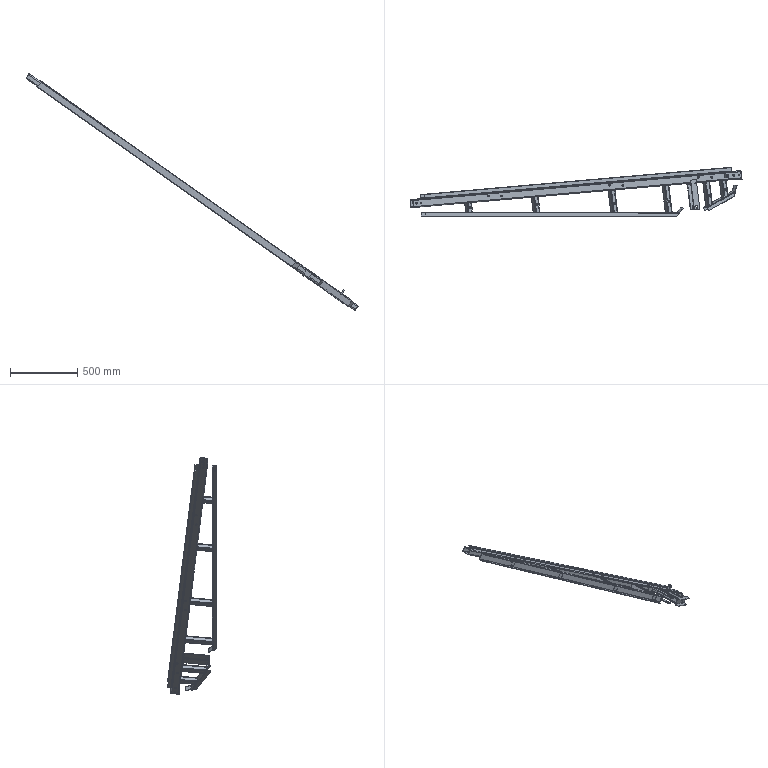Part | STEP file | HL4GZ-1.862.047 (left cane-feed mechanism frame) | 15 solids | 269 faces | box 2465 x 363.176 x 1756 mm | volume 3798659 mm3 | plane 154 | cylinder 115 | commonest cylinder face diameters 12 x32 6 x24 13 x24 10 x12 4 x8 14 x6